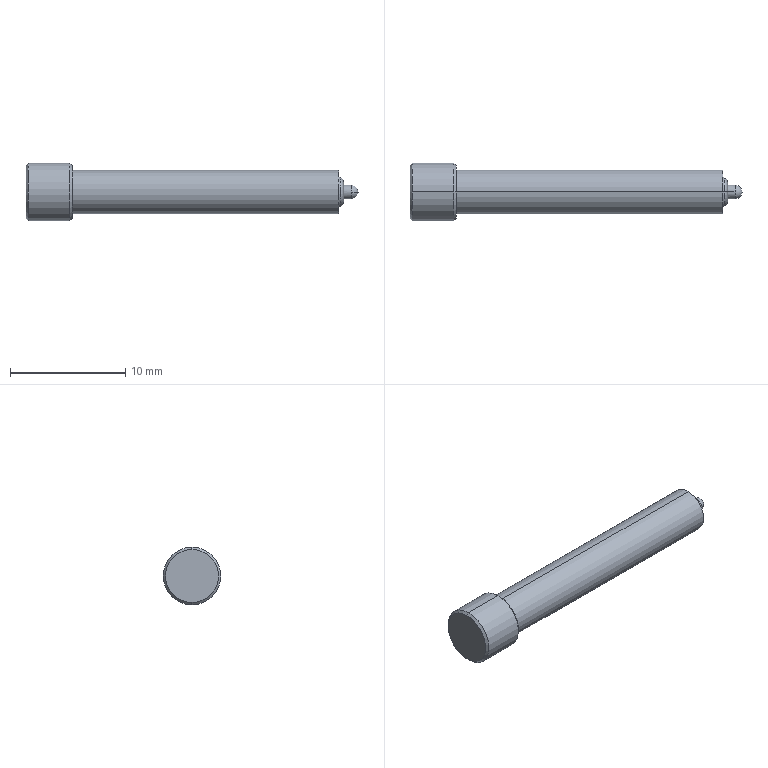Part | STEP file | Riveting punch | 1 solid | 20 faces | box 28.754 x 5 x 5 mm | volume 342.473 mm3 | cylinder 6 | torus 4 | cone 4 | plane 4 | sphere 2 | commonest cylinder face diameters 1.2 x2 3.8 x2 5 x2
STEP:
#1=CARTESIAN_POINT('',(0.,0.,0.));
#2=DIRECTION('',(0.,0.,1.));
#3=DIRECTION('',(1.,0.,0.));
#4=AXIS2_PLACEMENT_3D('',#1,#2,#3);
#5=CARTESIAN_POINT('',(17378.872,34.388,-1.214));
#6=VERTEX_POINT('',#5);
#7=CARTESIAN_POINT('',(17378.72,34.388,-1.85));
#8=VERTEX_POINT('',#7);
#9=CARTESIAN_POINT('',(17379.02,34.388,-1.585));
#10=DIRECTION('',(0.,-1.,0.));
#11=DIRECTION('',(0.,0.,-1.));
#12=AXIS2_PLACEMENT_3D('',#9,#10,#11);
#13=CIRCLE('',#12,0.4);
#14=CARTESIAN_POINT('',(17379.02,34.388,0.));
#15=DIRECTION('',(1.,0.,0.));
#16=DIRECTION('',(0.,0.,-1.));
#17=AXIS2_PLACEMENT_3D('',#14,#15,#16);
#18=TOROIDAL_SURFACE('',#17,1.585,0.4);
#19=CARTESIAN_POINT('',(6.283,0.));
#20=DIRECTION('',(0.,1.));
#21=VECTOR('',#20,1.);
#22=LINE('',#19,#21);
#23=(GEOMETRIC_REPRESENTATION_CONTEXT(2)PARAMETRIC_REPRESENTATION_CONTEXT()REPRESENTATION_CONTEXT('',''));
#24=DEFINITIONAL_REPRESENTATION('',(#22),#23);
#25=PCURVE('',#18,#24);
#26=CARTESIAN_POINT('',(17379.02,34.388,0.));
#27=DIRECTION('',(1.,0.,0.));
#28=DIRECTION('',(0.,0.,-1.));
#29=AXIS2_PLACEMENT_3D('',#26,#27,#28);
#30=TOROIDAL_SURFACE('',#29,1.585,0.4);
#31=CARTESIAN_POINT('',(0.,0.));
#32=DIRECTION('',(0.,1.));
#33=VECTOR('',#32,1.);
#34=LINE('',#31,#33);
#35=(GEOMETRIC_REPRESENTATION_CONTEXT(2)PARAMETRIC_REPRESENTATION_CONTEXT()REPRESENTATION_CONTEXT('',''));
#36=DEFINITIONAL_REPRESENTATION('',(#34),#35);
#37=PCURVE('',#30,#36);
#38=SURFACE_CURVE('',#13,(#25,#37),.PCURVE_S1.);
#39=EDGE_CURVE('',#6,#8,#38,.T.);
#40=ORIENTED_EDGE('',*,*,#39,.T.);
#41=CARTESIAN_POINT('',(17378.72,34.388,1.85));
#42=VERTEX_POINT('',#41);
#43=CARTESIAN_POINT('',(17378.72,34.388,0.));
#44=DIRECTION('',(1.,0.,0.));
#45=DIRECTION('',(0.,0.,-1.));
#46=AXIS2_PLACEMENT_3D('',#43,#44,#45);
#47=CIRCLE('',#46,1.85);
#48=CARTESIAN_POINT('',(0.,5.435));
#49=DIRECTION('',(1.,0.));
#50=VECTOR('',#49,1.);
#51=LINE('',#48,#50);
#52=(GEOMETRIC_REPRESENTATION_CONTEXT(2)PARAMETRIC_REPRESENTATION_CONTEXT()REPRESENTATION_CONTEXT('',''));
#53=DEFINITIONAL_REPRESENTATION('',(#51),#52);
#54=PCURVE('',#18,#53);
#55=CARTESIAN_POINT('',(17378.72,36.238,0.));
#56=DIRECTION('',(1.,0.,0.));
#57=DIRECTION('',(0.,0.,-1.));
#58=AXIS2_PLACEMENT_3D('',#55,#56,#57);
#59=PLANE('',#58);
#60=CARTESIAN_POINT('',(0.,-1.85));
#61=DIRECTION('',(1.,0.));
#62=AXIS2_PLACEMENT_2D('',#60,#61);
#63=CIRCLE('',#62,1.85);
#64=(GEOMETRIC_REPRESENTATION_CONTEXT(2)PARAMETRIC_REPRESENTATION_CONTEXT()REPRESENTATION_CONTEXT('',''));
#65=DEFINITIONAL_REPRESENTATION('',(#63),#64);
#66=PCURVE('',#59,#65);
#67=SURFACE_CURVE('',#47,(#54,#66),.PCURVE_S1.);
#68=EDGE_CURVE('',#42,#8,#67,.T.);
#69=ORIENTED_EDGE('',*,*,#68,.F.);
#70=CARTESIAN_POINT('',(17378.872,34.388,1.214));
#71=VERTEX_POINT('',#70);
#72=CARTESIAN_POINT('',(17379.02,34.388,1.585));
#73=DIRECTION('',(0.,1.,0.));
#74=DIRECTION('',(0.,0.,1.));
#75=AXIS2_PLACEMENT_3D('',#72,#73,#74);
#76=CIRCLE('',#75,0.4);
#77=CARTESIAN_POINT('',(3.142,0.));
#78=DIRECTION('',(0.,1.));
#79=VECTOR('',#78,1.);
#80=LINE('',#77,#79);
#81=(GEOMETRIC_REPRESENTATION_CONTEXT(2)PARAMETRIC_REPRESENTATION_CONTEXT()REPRESENTATION_CONTEXT('',''));
#82=DEFINITIONAL_REPRESENTATION('',(#80),#81);
#83=PCURVE('',#18,#82);
#84=CARTESIAN_POINT('',(3.142,0.));
#85=DIRECTION('',(0.,1.));
#86=VECTOR('',#85,1.);
#87=LINE('',#84,#86);
#88=(GEOMETRIC_REPRESENTATION_CONTEXT(2)PARAMETRIC_REPRESENTATION_CONTEXT()REPRESENTATION_CONTEXT('',''));
#89=DEFINITIONAL_REPRESENTATION('',(#87),#88);
#90=PCURVE('',#30,#89);
#91=SURFACE_CURVE('',#76,(#83,#90),.PCURVE_S1.);
#92=EDGE_CURVE('',#71,#42,#91,.T.);
#93=ORIENTED_EDGE('',*,*,#92,.F.);
#94=CARTESIAN_POINT('',(17378.872,34.388,0.));
#95=DIRECTION('',(1.,0.,0.));
#96=DIRECTION('',(0.,0.,-1.));
#97=AXIS2_PLACEMENT_3D('',#94,#95,#96);
#98=CIRCLE('',#97,1.214);
#99=CARTESIAN_POINT('',(0.,3.521));
#100=DIRECTION('',(1.,0.));
#101=VECTOR('',#100,1.);
#102=LINE('',#99,#101);
#103=(GEOMETRIC_REPRESENTATION_CONTEXT(2)PARAMETRIC_REPRESENTATION_CONTEXT()REPRESENTATION_CONTEXT('',''));
#104=DEFINITIONAL_REPRESENTATION('',(#102),#103);
#105=PCURVE('',#18,#104);
#106=CARTESIAN_POINT('',(17378.723,34.388,0.));
#107=DIRECTION('',(1.,0.,0.));
#108=DIRECTION('',(0.,0.,-1.));
#109=AXIS2_PLACEMENT_3D('',#106,#107,#108);
#110=TOROIDAL_SURFACE('',#109,0.8424,0.4);
#111=CARTESIAN_POINT('',(0.,0.3796));
#112=DIRECTION('',(1.,0.));
#113=VECTOR('',#112,1.);
#114=LINE('',#111,#113);
#115=(GEOMETRIC_REPRESENTATION_CONTEXT(2)PARAMETRIC_REPRESENTATION_CONTEXT()REPRESENTATION_CONTEXT('',''));
#116=DEFINITIONAL_REPRESENTATION('',(#114),#115);
#117=PCURVE('',#110,#116);
#118=SURFACE_CURVE('',#98,(#105,#117),.PCURVE_S1.);
#119=EDGE_CURVE('',#71,#6,#118,.T.);
#120=ORIENTED_EDGE('',*,*,#119,.T.);
#121=EDGE_LOOP('',(#40,#69,#93,#120));
#122=FACE_BOUND('',#121,.F.);
#123=ADVANCED_FACE('',(#122),#18,.F.);
#124=CARTESIAN_POINT('',(17378.872,34.388,0.));
#125=DIRECTION('',(1.,0.,0.));
#126=DIRECTION('',(0.,0.,-1.));
#127=AXIS2_PLACEMENT_3D('',#124,#125,#126);
#128=CIRCLE('',#127,1.214);
#129=CARTESIAN_POINT('',(17378.723,34.388,0.));
#130=DIRECTION('',(1.,0.,0.));
#131=DIRECTION('',(0.,0.,-1.));
#132=AXIS2_PLACEMENT_3D('',#129,#130,#131);
#133=TOROIDAL_SURFACE('',#132,0.8424,0.4);
#134=CARTESIAN_POINT('',(0.,0.3796));
#135=DIRECTION('',(1.,0.));
#136=VECTOR('',#135,1.);
#137=LINE('',#134,#136);
#138=(GEOMETRIC_REPRESENTATION_CONTEXT(2)PARAMETRIC_REPRESENTATION_CONTEXT()REPRESENTATION_CONTEXT('',''));
#139=DEFINITIONAL_REPRESENTATION('',(#137),#138);
#140=PCURVE('',#133,#139);
#141=CARTESIAN_POINT('',(0.,3.521));
#142=DIRECTION('',(1.,0.));
#143=VECTOR('',#142,1.);
#144=LINE('',#141,#143);
#145=(GEOMETRIC_REPRESENTATION_CONTEXT(2)PARAMETRIC_REPRESENTATION_CONTEXT()REPRESENTATION_CONTEXT('',''));
#146=DEFINITIONAL_REPRESENTATION('',(#144),#145);
#147=PCURVE('',#30,#146);
#148=SURFACE_CURVE('',#128,(#140,#147),.PCURVE_S1.);
#149=EDGE_CURVE('',#6,#71,#148,.T.);
#150=ORIENTED_EDGE('',*,*,#149,.T.);
#151=CARTESIAN_POINT('',(17379.123,34.388,0.8424));
#152=VERTEX_POINT('',#151);
#153=CARTESIAN_POINT('',(17378.723,34.388,0.8424));
#154=DIRECTION('',(0.,1.,0.));
#155=DIRECTION('',(0.,0.,1.));
#156=AXIS2_PLACEMENT_3D('',#153,#154,#155);
#157=CIRCLE('',#156,0.4);
#158=CARTESIAN_POINT('',(3.142,0.));
#159=DIRECTION('',(0.,1.));
#160=VECTOR('',#159,1.);
#161=LINE('',#158,#160);
#162=(GEOMETRIC_REPRESENTATION_CONTEXT(2)PARAMETRIC_REPRESENTATION_CONTEXT()REPRESENTATION_CONTEXT('',''));
#163=DEFINITIONAL_REPRESENTATION('',(#161),#162);
#164=PCURVE('',#133,#163);
#165=CARTESIAN_POINT('',(3.142,0.));
#166=DIRECTION('',(0.,1.));
#167=VECTOR('',#166,1.);
#168=LINE('',#165,#167);
#169=(GEOMETRIC_REPRESENTATION_CONTEXT(2)PARAMETRIC_REPRESENTATION_CONTEXT()REPRESENTATION_CONTEXT('',''));
#170=DEFINITIONAL_REPRESENTATION('',(#168),#169);
#171=PCURVE('',#110,#170);
#172=SURFACE_CURVE('',#157,(#164,#171),.PCURVE_S1.);
#173=EDGE_CURVE('',#71,#152,#172,.T.);
#174=ORIENTED_EDGE('',*,*,#173,.T.);
#175=CARTESIAN_POINT('',(17379.123,34.388,-0.8424));
#176=VERTEX_POINT('',#175);
#177=CARTESIAN_POINT('',(17379.123,34.388,0.));
#178=DIRECTION('',(1.,0.,0.));
#179=DIRECTION('',(0.,0.,-1.));
#180=AXIS2_PLACEMENT_3D('',#177,#178,#179);
#181=CIRCLE('',#180,0.8424);
#182=CARTESIAN_POINT('',(0.,1.571));
#183=DIRECTION('',(1.,0.));
#184=VECTOR('',#183,1.);
#185=LINE('',#182,#184);
#186=(GEOMETRIC_REPRESENTATION_CONTEXT(2)PARAMETRIC_REPRESENTATION_CONTEXT()REPRESENTATION_CONTEXT('',''));
#187=DEFINITIONAL_REPRESENTATION('',(#185),#186);
#188=PCURVE('',#133,#187);
#189=CARTESIAN_POINT('',(17379.123,35.231,0.));
#190=DIRECTION('',(1.,0.,0.));
#191=DIRECTION('',(0.,0.,-1.));
#192=AXIS2_PLACEMENT_3D('',#189,#190,#191);
#193=PLANE('',#192);
#194=CARTESIAN_POINT('',(0.,-0.8424));
#195=DIRECTION('',(1.,0.));
#196=AXIS2_PLACEMENT_2D('',#194,#195);
#197=CIRCLE('',#196,0.8424);
#198=(GEOMETRIC_REPRESENTATION_CONTEXT(2)PARAMETRIC_REPRESENTATION_CONTEXT()REPRESENTATION_CONTEXT('',''));
#199=DEFINITIONAL_REPRESENTATION('',(#197),#198);
#200=PCURVE('',#193,#199);
#201=SURFACE_CURVE('',#181,(#188,#200),.PCURVE_S1.);
#202=EDGE_CURVE('',#176,#152,#201,.T.);
#203=ORIENTED_EDGE('',*,*,#202,.F.);
#204=CARTESIAN_POINT('',(17378.723,34.388,-0.8424));
#205=DIRECTION('',(0.,-1.,0.));
#206=DIRECTION('',(0.,0.,-1.));
#207=AXIS2_PLACEMENT_3D('',#204,#205,#206);
#208=CIRCLE('',#207,0.4);
#209=CARTESIAN_POINT('',(0.,0.));
#210=DIRECTION('',(0.,1.));
#211=VECTOR('',#210,1.);
#212=LINE('',#209,#211);
#213=(GEOMETRIC_REPRESENTATION_CONTEXT(2)PARAMETRIC_REPRESENTATION_CONTEXT()REPRESENTATION_CONTEXT('',''));
#214=DEFINITIONAL_REPRESENTATION('',(#212),#213);
#215=PCURVE('',#133,#214);
#216=CARTESIAN_POINT('',(6.283,0.));
#217=DIRECTION('',(0.,1.));
#218=VECTOR('',#217,1.);
#219=LINE('',#216,#218);
#220=(GEOMETRIC_REPRESENTATION_CONTEXT(2)PARAMETRIC_REPRESENTATION_CONTEXT()REPRESENTATION_CONTEXT('',''));
#221=DEFINITIONAL_REPRESENTATION('',(#219),#220);
#222=PCURVE('',#110,#221);
#223=SURFACE_CURVE('',#208,(#215,#222),.PCURVE_S1.);
#224=EDGE_CURVE('',#6,#176,#223,.T.);
#225=ORIENTED_EDGE('',*,*,#224,.F.);
#226=EDGE_LOOP('',(#150,#174,#203,#225));
#227=FACE_BOUND('',#226,.T.);
#228=ADVANCED_FACE('',(#227),#133,.T.);
#229=CARTESIAN_POINT('',(17379.123,34.388,-0.6));
#230=VERTEX_POINT('',#229);
#231=CARTESIAN_POINT('',(17379.123,34.388,0.6));
#232=VERTEX_POINT('',#231);
#233=CARTESIAN_POINT('',(17379.123,34.388,0.));
#234=DIRECTION('',(1.,0.,0.));
#235=DIRECTION('',(0.,0.,-1.));
#236=AXIS2_PLACEMENT_3D('',#233,#234,#235);
#237=CIRCLE('',#236,0.6);
#238=CARTESIAN_POINT('',(17380.373,34.388,0.));
#239=DIRECTION('',(1.,0.,0.));
#240=DIRECTION('',(0.,0.,-1.));
#241=AXIS2_PLACEMENT_3D('',#238,#239,#240);
#242=CYLINDRICAL_SURFACE('',#241,0.6);
#243=CARTESIAN_POINT('',(0.,-1.25));
#244=DIRECTION('',(1.,0.));
#245=VECTOR('',#244,1.);
#246=LINE('',#243,#245);
#247=(GEOMETRIC_REPRESENTATION_CONTEXT(2)PARAMETRIC_REPRESENTATION_CONTEXT()REPRESENTATION_CONTEXT('',''));
#248=DEFINITIONAL_REPRESENTATION('',(#246),#247);
#249=PCURVE('',#242,#248);
#250=CARTESIAN_POINT('',(0.,-0.8424));
#251=DIRECTION('',(1.,0.));
#252=AXIS2_PLACEMENT_2D('',#250,#251);
#253=CIRCLE('',#252,0.6);
#254=(GEOMETRIC_REPRESENTATION_CONTEXT(2)PARAMETRIC_REPRESENTATION_CONTEXT()REPRESENTATION_CONTEXT('',''));
#255=DEFINITIONAL_REPRESENTATION('',(#253),#254);
#256=PCURVE('',#193,#255);
#257=SURFACE_CURVE('',#237,(#249,#256),.PCURVE_S1.);
#258=EDGE_CURVE('',#230,#232,#257,.T.);
#259=ORIENTED_EDGE('',*,*,#258,.T.);
#260=CARTESIAN_POINT('',(17379.773,34.388,0.6));
#261=VERTEX_POINT('',#260);
#262=CARTESIAN_POINT('',(17380.373,34.388,0.6));
#263=DIRECTION('',(1.,0.,0.));
#264=VECTOR('',#263,1.);
#265=LINE('',#262,#264);
#266=CARTESIAN_POINT('',(3.142,0.));
#267=DIRECTION('',(0.,1.));
#268=VECTOR('',#267,1.);
#269=LINE('',#266,#268);
#270=(GEOMETRIC_REPRESENTATION_CONTEXT(2)PARAMETRIC_REPRESENTATION_CONTEXT()REPRESENTATION_CONTEXT('',''));
#271=DEFINITIONAL_REPRESENTATION('',(#269),#270);
#272=PCURVE('',#242,#271);
#273=CARTESIAN_POINT('',(17380.373,34.388,0.));
#274=DIRECTION('',(1.,0.,0.));
#275=DIRECTION('',(0.,0.,-1.));
#276=AXIS2_PLACEMENT_3D('',#273,#274,#275);
#277=CYLINDRICAL_SURFACE('',#276,0.6);
#278=CARTESIAN_POINT('',(3.142,0.));
#279=DIRECTION('',(0.,1.));
#280=VECTOR('',#279,1.);
#281=LINE('',#278,#280);
#282=(GEOMETRIC_REPRESENTATION_CONTEXT(2)PARAMETRIC_REPRESENTATION_CONTEXT()REPRESENTATION_CONTEXT('',''));
#283=DEFINITIONAL_REPRESENTATION('',(#281),#282);
#284=PCURVE('',#277,#283);
#285=SURFACE_CURVE('',#265,(#272,#284),.PCURVE_S1.);
#286=EDGE_CURVE('',#232,#261,#285,.T.);
#287=ORIENTED_EDGE('',*,*,#286,.T.);
#288=CARTESIAN_POINT('',(17379.773,34.988,0.));
#289=VERTEX_POINT('',#288);
#290=CARTESIAN_POINT('',(17379.773,34.388,0.));
#291=DIRECTION('',(1.,0.,0.));
#292=DIRECTION('',(0.,0.,-1.));
#293=AXIS2_PLACEMENT_3D('',#290,#291,#292);
#294=CIRCLE('',#293,0.6);
#295=CARTESIAN_POINT('',(0.,-0.6));
#296=DIRECTION('',(1.,0.));
#297=VECTOR('',#296,1.);
#298=LINE('',#295,#297);
#299=(GEOMETRIC_REPRESENTATION_CONTEXT(2)PARAMETRIC_REPRESENTATION_CONTEXT()REPRESENTATION_CONTEXT('',''));
#300=DEFINITIONAL_REPRESENTATION('',(#298),#299);
#301=PCURVE('',#242,#300);
#302=CARTESIAN_POINT('',(17379.773,34.388,0.));
#303=DIRECTION('',(0.,0.,1.));
#304=DIRECTION('',(0.,1.,0.));
#305=AXIS2_PLACEMENT_3D('',#302,#303,#304);
#306=SPHERICAL_SURFACE('',#305,0.6);
#307=CARTESIAN_POINT('',(6.283,-1.571));
#308=DIRECTION('',(0.,1.));
#309=VECTOR('',#308,1.);
#310=LINE('',#307,#309);
#311=(GEOMETRIC_REPRESENTATION_CONTEXT(2)PARAMETRIC_REPRESENTATION_CONTEXT()REPRESENTATION_CONTEXT('',''));
#312=DEFINITIONAL_REPRESENTATION('',(#310),#311);
#313=PCURVE('',#306,#312);
#314=SURFACE_CURVE('',#294,(#301,#313),.PCURVE_S1.);
#315=EDGE_CURVE('',#289,#261,#314,.T.);
#316=ORIENTED_EDGE('',*,*,#315,.F.);
#317=CARTESIAN_POINT('',(17379.773,34.388,-0.6));
#318=VERTEX_POINT('',#317);
#319=CARTESIAN_POINT('',(17379.773,34.388,0.));
#320=DIRECTION('',(1.,0.,0.));
#321=DIRECTION('',(0.,0.,-1.));
#322=AXIS2_PLACEMENT_3D('',#319,#320,#321);
#323=CIRCLE('',#322,0.6);
#324=CARTESIAN_POINT('',(0.,-0.6));
#325=DIRECTION('',(1.,0.));
#326=VECTOR('',#325,1.);
#327=LINE('',#324,#326);
#328=(GEOMETRIC_REPRESENTATION_CONTEXT(2)PARAMETRIC_REPRESENTATION_CONTEXT()REPRESENTATION_CONTEXT('',''));
#329=DEFINITIONAL_REPRESENTATION('',(#327),#328);
#330=PCURVE('',#242,#329);
#331=CARTESIAN_POINT('',(17379.773,34.388,0.));
#332=DIRECTION('',(0.,0.,1.));
#333=DIRECTION('',(0.,1.,0.));
#334=AXIS2_PLACEMENT_3D('',#331,#332,#333);
#335=SPHERICAL_SURFACE('',#334,0.6);
#336=CARTESIAN_POINT('',(6.283,-1.571));
#337=DIRECTION('',(0.,1.));
#338=VECTOR('',#337,1.);
#339=LINE('',#336,#338);
#340=(GEOMETRIC_REPRESENTATION_CONTEXT(2)PARAMETRIC_REPRESENTATION_CONTEXT()REPRESENTATION_CONTEXT('',''));
#341=DEFINITIONAL_REPRESENTATION('',(#339),#340);
#342=PCURVE('',#335,#341);
#343=SURFACE_CURVE('',#323,(#330,#342),.PCURVE_S1.);
#344=EDGE_CURVE('',#318,#289,#343,.T.);
#345=ORIENTED_EDGE('',*,*,#344,.F.);
#346=CARTESIAN_POINT('',(17380.373,34.388,-0.6));
#347=DIRECTION('',(1.,0.,0.));
#348=VECTOR('',#347,1.);
#349=LINE('',#346,#348);
#350=CARTESIAN_POINT('',(0.,0.));
#351=DIRECTION('',(0.,1.));
#352=VECTOR('',#351,1.);
#353=LINE('',#350,#352);
#354=(GEOMETRIC_REPRESENTATION_CONTEXT(2)PARAMETRIC_REPRESENTATION_CONTEXT()REPRESENTATION_CONTEXT('',''));
#355=DEFINITIONAL_REPRESENTATION('',(#353),#354);
#356=PCURVE('',#242,#355);
#357=CARTESIAN_POINT('',(6.283,0.));
#358=DIRECTION('',(0.,1.));
#359=VECTOR('',#358,1.);
#360=LINE('',#357,#359);
#361=(GEOMETRIC_REPRESENTATION_CONTEXT(2)PARAMETRIC_REPRESENTATION_CONTEXT()REPRESENTATION_CONTEXT('',''));
#362=DEFINITIONAL_REPRESENTATION('',(#360),#361);
#363=PCURVE('',#277,#362);
#364=SURFACE_CURVE('',#349,(#356,#363),.PCURVE_S1.);
#365=EDGE_CURVE('',#230,#318,#364,.T.);
#366=ORIENTED_EDGE('',*,*,#365,.F.);
#367=EDGE_LOOP('',(#259,#287,#316,#345,#366));
#368=FACE_BOUND('',#367,.T.);
#369=ADVANCED_FACE('',(#368),#242,.T.);
#370=ORIENTED_EDGE('',*,*,#315,.T.);
#371=CARTESIAN_POINT('',(17379.773,33.788,0.));
#372=VERTEX_POINT('',#371);
#373=CARTESIAN_POINT('',(17379.773,34.388,0.));
#374=DIRECTION('',(1.,0.,0.));
#375=DIRECTION('',(0.,0.,-1.));
#376=AXIS2_PLACEMENT_3D('',#373,#374,#375);
#377=CIRCLE('',#376,0.6);
#378=CARTESIAN_POINT('',(3.142,1.571));
#379=CARTESIAN_POINT('',(3.142,1.547));
#380=CARTESIAN_POINT('',(3.142,1.499));
#381=CARTESIAN_POINT('',(3.142,1.428));
#382=CARTESIAN_POINT('',(3.142,1.357));
#383=CARTESIAN_POINT('',(3.142,1.285));
#384=CARTESIAN_POINT('',(3.142,1.214));
#385=CARTESIAN_POINT('',(3.142,1.142));
#386=CARTESIAN_POINT('',(3.142,1.071));
#387=CARTESIAN_POINT('',(3.142,0.9996));
#388=CARTESIAN_POINT('',(3.142,0.9282));
#389=CARTESIAN_POINT('',(3.142,0.8568));
#390=CARTESIAN_POINT('',(3.142,0.7854));
#391=CARTESIAN_POINT('',(3.142,0.714));
#392=CARTESIAN_POINT('',(3.142,0.6426));
#393=CARTESIAN_POINT('',(3.142,0.5712));
#394=CARTESIAN_POINT('',(3.142,0.4998));
#395=CARTESIAN_POINT('',(3.142,0.4284));
#396=CARTESIAN_POINT('',(3.142,0.357));
#397=CARTESIAN_POINT('',(3.142,0.2856));
#398=CARTESIAN_POINT('',(3.142,0.2142));
#399=CARTESIAN_POINT('',(3.142,0.1428));
#400=CARTESIAN_POINT('',(3.142,0.0714));
#401=CARTESIAN_POINT('',(3.142,0.0238));
#402=CARTESIAN_POINT('',(3.142,0.));
#403=B_SPLINE_CURVE_WITH_KNOTS('',3,(#378,#379,#380,#381,#382,#383,#384,#385,#386,#387,#388,#389,#390,#391,#392,#393,#394,#395,#396,#397,#398,#399,#400,#401,#402),.UNSPECIFIED.,.F.,.F.,(4,1,1,1,1,1,1,1,1,1,1,1,1,1,1,1,1,1,1,1,1,1,4),(3.142,3.213,3.284,3.356,3.427,3.499,3.57,3.641,3.713,3.784,3.856,3.927,3.998,4.07,4.141,4.213,4.284,4.355,4.427,4.498,4.57,4.641,4.712),.QUASI_UNIFORM_KNOTS.);
#404=(GEOMETRIC_REPRESENTATION_CONTEXT(2)PARAMETRIC_REPRESENTATION_CONTEXT()REPRESENTATION_CONTEXT('',''));
#405=DEFINITIONAL_REPRESENTATION('',(#403),#404);
#406=PCURVE('',#306,#405);
#407=CARTESIAN_POINT('',(0.,-0.6));
#408=DIRECTION('',(1.,0.));
#409=VECTOR('',#408,1.);
#410=LINE('',#407,#409);
#411=(GEOMETRIC_REPRESENTATION_CONTEXT(2)PARAMETRIC_REPRESENTATION_CONTEXT()REPRESENTATION_CONTEXT('',''));
#412=DEFINITIONAL_REPRESENTATION('',(#410),#411);
#413=PCURVE('',#277,#412);
#414=SURFACE_CURVE('',#377,(#406,#413),.PCURVE_S1.);
#415=EDGE_CURVE('',#261,#372,#414,.T.);
#416=ORIENTED_EDGE('',*,*,#415,.T.);
#417=CARTESIAN_POINT('',(17380.373,34.388,0.));
#418=VERTEX_POINT('',#417);
#419=CARTESIAN_POINT('',(17379.773,34.388,0.));
#420=DIRECTION('',(0.,0.,1.));
#421=DIRECTION('',(0.,-1.,0.));
#422=AXIS2_PLACEMENT_3D('',#419,#420,#421);
#423=CIRCLE('',#422,0.6);
#424=CARTESIAN_POINT('',(3.142,0.));
#425=DIRECTION('',(1.,0.));
#426=VECTOR('',#425,1.);
#427=LINE('',#424,#426);
#428=(GEOMETRIC_REPRESENTATION_CONTEXT(2)PARAMETRIC_REPRESENTATION_CONTEXT()REPRESENTATION_CONTEXT('',''));
#429=DEFINITIONAL_REPRESENTATION('',(#427),#428);
#430=PCURVE('',#306,#429);
#431=CARTESIAN_POINT('',(3.142,0.));
#432=DIRECTION('',(1.,0.));
#433=VECTOR('',#432,1.);
#434=LINE('',#431,#433);
#435=(GEOMETRIC_REPRESENTATION_CONTEXT(2)PARAMETRIC_REPRESENTATION_CONTEXT()REPRESENTATION_CONTEXT('',''));
#436=DEFINITIONAL_REPRESENTATION('',(#434),#435);
#437=PCURVE('',#335,#436);
#438=SURFACE_CURVE('',#423,(#430,#437),.PCURVE_S1.);
#439=EDGE_CURVE('',#372,#418,#438,.T.);
#440=ORIENTED_EDGE('',*,*,#439,.T.);
#441=CARTESIAN_POINT('',(17379.773,34.388,0.));
#442=DIRECTION('',(0.,0.,-1.));
#443=DIRECTION('',(-1.,0.,0.));
#444=AXIS2_PLACEMENT_3D('',#441,#442,#443);
#445=CIRCLE('',#444,0.6);
#446=CARTESIAN_POINT('',(6.283,0.));
#447=CARTESIAN_POINT('',(6.259,0.));
#448=CARTESIAN_POINT('',(6.212,0.));
#449=CARTESIAN_POINT('',(6.14,0.));
#450=CARTESIAN_POINT('',(6.069,0.));
#451=CARTESIAN_POINT('',(5.998,0.));
#452=CARTESIAN_POINT('',(5.926,0.));
#453=CARTESIAN_POINT('',(5.855,0.));
#454=CARTESIAN_POINT('',(5.783,0.));
#455=CARTESIAN_POINT('',(5.712,0.));
#456=CARTESIAN_POINT('',(5.641,0.));
#457=CARTESIAN_POINT('',(5.569,0.));
#458=CARTESIAN_POINT('',(5.498,0.));
#459=CARTESIAN_POINT('',(5.426,0.));
#460=CARTESIAN_POINT('',(5.355,0.));
#461=CARTESIAN_POINT('',(5.284,0.));
#462=CARTESIAN_POINT('',(5.212,0.));
#463=CARTESIAN_POINT('',(5.141,0.));
#464=CARTESIAN_POINT('',(5.069,0.));
#465=CARTESIAN_POINT('',(4.998,0.));
#466=CARTESIAN_POINT('',(4.927,0.));
#467=CARTESIAN_POINT('',(4.855,0.));
#468=CARTESIAN_POINT('',(4.784,0.));
#469=CARTESIAN_POINT('',(4.736,0.));
#470=CARTESIAN_POINT('',(4.712,0.));
#471=B_SPLINE_CURVE_WITH_KNOTS('',3,(#446,#447,#448,#449,#450,#451,#452,#453,#454,#455,#456,#457,#458,#459,#460,#461,#462,#463,#464,#465,#466,#467,#468,#469,#470),.UNSPECIFIED.,.F.,.F.,(4,1,1,1,1,1,1,1,1,1,1,1,1,1,1,1,1,1,1,1,1,1,4),(1.571,1.642,1.714,1.785,1.856,1.928,1.999,2.071,2.142,2.213,2.285,2.356,2.428,2.499,2.57,2.642,2.713,2.785,2.856,2.927,2.999,3.07,3.142),.QUASI_UNIFORM_KNOTS.);
#472=(GEOMETRIC_REPRESENTATION_CONTEXT(2)PARAMETRIC_REPRESENTATION_CONTEXT()REPRESENTATION_CONTEXT('',''));
#473=DEFINITIONAL_REPRESENTATION('',(#471),#472);
#474=PCURVE('',#306,#473);
#475=CARTESIAN_POINT('',(6.283,0.));
#476=CARTESIAN_POINT('',(6.259,0.));
#477=CARTESIAN_POINT('',(6.212,0.));
#478=CARTESIAN_POINT('',(6.14,0.));
#479=CARTESIAN_POINT('',(6.069,0.));
#480=CARTESIAN_POINT('',(5.998,0.));
#481=CARTESIAN_POINT('',(5.926,0.));
#482=CARTESIAN_POINT('',(5.855,0.));
#483=CARTESIAN_POINT('',(5.783,0.));
#484=CARTESIAN_POINT('',(5.712,0.));
#485=CARTESIAN_POINT('',(5.641,0.));
#486=CARTESIAN_POINT('',(5.569,0.));
#487=CARTESIAN_POINT('',(5.498,0.));
#488=CARTESIAN_POINT('',(5.426,0.));
#489=CARTESIAN_POINT('',(5.355,0.));
#490=CARTESIAN_POINT('',(5.284,0.));
#491=CARTESIAN_POINT('',(5.212,0.));
#492=CARTESIAN_POINT('',(5.141,0.));
#493=CARTESIAN_POINT('',(5.069,0.));
#494=CARTESIAN_POINT('',(4.998,0.));
#495=CARTESIAN_POINT('',(4.927,0.));
#496=CARTESIAN_POINT('',(4.855,0.));
#497=CARTESIAN_POINT('',(4.784,0.));
#498=CARTESIAN_POINT('',(4.736,0.));
#499=CARTESIAN_POINT('',(4.712,0.));
#500=B_SPLINE_CURVE_WITH_KNOTS('',3,(#475,#476,#477,#478,#479,#480,#481,#482,#483,#484,#485,#486,#487,#488,#489,#490,#491,#492,#493,#494,#495,#496,#497,#498,#499),.UNSPECIFIED.,.F.,.F.,(4,1,1,1,1,1,1,1,1,1,1,1,1,1,1,1,1,1,1,1,1,1,4),(1.571,1.642,1.714,1.785,1.856,1.928,1.999,2.071,2.142,2.213,2.285,2.356,2.428,2.499,2.57,2.642,2.713,2.785,2.856,2.927,2.999,3.07,3.142),.QUASI_UNIFORM_KNOTS.);
#501=(GEOMETRIC_REPRESENTATION_CONTEXT(2)PARAMETRIC_REPRESENTATION_CONTEXT()REPRESENTATION_CONTEXT('',''));
#502=DEFINITIONAL_REPRESENTATION('',(#500),#501);
#503=PCURVE('',#335,#502);
#504=SURFACE_CURVE('',#445,(#474,#503),.PCURVE_S1.);
#505=EDGE_CURVE('',#289,#418,#504,.T.);
#506=ORIENTED_EDGE('',*,*,#505,.F.);
#507=EDGE_LOOP('',(#370,#416,#440,#506));
#508=FACE_BOUND('',#507,.T.);
#509=ADVANCED_FACE('',(#508),#306,.T.);
#510=CARTESIAN_POINT('',(17351.62,34.388,-2.3));
#511=VERTEX_POINT('',#510);
#512=CARTESIAN_POINT('',(17351.62,34.388,2.3));
#513=VERTEX_POINT('',#512);
#514=CARTESIAN_POINT('',(17351.62,34.388,0.));
#515=DIRECTION('',(1.,0.,0.));
#516=DIRECTION('',(0.,0.,-1.));
#517=AXIS2_PLACEMENT_3D('',#514,#515,#516);
#518=CIRCLE('',#517,2.3);
#519=CARTESIAN_POINT('',(17351.82,34.388,0.));
#520=DIRECTION('',(1.,0.,0.));
#521=DIRECTION('',(0.,0.,-1.));
#522=AXIS2_PLACEMENT_3D('',#519,#520,#521);
#523=CONICAL_SURFACE('',#522,2.5,0.7854);
#524=CARTESIAN_POINT('',(0.,-0.2));
#525=DIRECTION('',(1.,0.));
#526=VECTOR('',#525,1.);
#527=LINE('',#524,#526);
#528=(GEOMETRIC_REPRESENTATION_CONTEXT(2)PARAMETRIC_REPRESENTATION_CONTEXT()REPRESENTATION_CONTEXT('',''));
#529=DEFINITIONAL_REPRESENTATION('',(#527),#528);
#530=PCURVE('',#523,#529);
#531=CARTESIAN_POINT('',(17351.62,36.688,0.));
#532=DIRECTION('',(-1.,0.,0.));
#533=DIRECTION('',(0.,0.,1.));
#534=AXIS2_PLACEMENT_3D('',#531,#532,#533);
#535=PLANE('',#534);
#536=CARTESIAN_POINT('',(-2.3,-2.3));
#537=CARTESIAN_POINT('',(-2.3,1.684));
#538=CARTESIAN_POINT('',(1.15,-0.3081));
#539=CARTESIAN_POINT('',(4.6,-2.3));
#540=CARTESIAN_POINT('',(1.15,-4.292));
#541=CARTESIAN_POINT('',(-2.3,-6.284));
#542=CARTESIAN_POINT('',(-2.3,-2.3));
#543=(BOUNDED_CURVE()B_SPLINE_CURVE(2,(#536,#537,#538,#539,#540,#541,#542),.UNSPECIFIED.,.T.,.F.)B_SPLINE_CURVE_WITH_KNOTS((1,2,2,2,2,1),(-2.094,0.,2.094,4.189,6.283,8.378),.UNSPECIFIED.)CURVE()GEOMETRIC_REPRESENTATION_ITEM()RATIONAL_B_SPLINE_CURVE((1.,0.5,1.,0.5,1.,0.5,1.))REPRESENTATION_ITEM(''));
#544=(GEOMETRIC_REPRESENTATION_CONTEXT(2)PARAMETRIC_REPRESENTATION_CONTEXT()REPRESENTATION_CONTEXT('',''));
#545=DEFINITIONAL_REPRESENTATION('',(#543),#544);
#546=PCURVE('',#535,#545);
#547=SURFACE_CURVE('',#518,(#530,#546),.PCURVE_S1.);
#548=EDGE_CURVE('',#511,#513,#547,.T.);
#549=ORIENTED_EDGE('',*,*,#548,.T.);
#550=CARTESIAN_POINT('',(17351.82,34.388,2.5));
#551=VERTEX_POINT('',#550);
#552=CARTESIAN_POINT('',(17351.82,34.388,2.5));
#553=DIRECTION('',(0.7071,0.,0.7071));
#554=VECTOR('',#553,1.);
#555=LINE('',#552,#554);
#556=CARTESIAN_POINT('',(3.142,0.));
#557=DIRECTION('',(0.,1.));
#558=VECTOR('',#557,1.);
#559=LINE('',#556,#558);
#560=(GEOMETRIC_REPRESENTATION_CONTEXT(2)PARAMETRIC_REPRESENTATION_CONTEXT()REPRESENTATION_CONTEXT('',''));
#561=DEFINITIONAL_REPRESENTATION('',(#559),#560);
#562=PCURVE('',#523,#561);
#563=CARTESIAN_POINT('',(17351.82,34.388,0.));
#564=DIRECTION('',(1.,0.,0.));
#565=DIRECTION('',(0.,0.,-1.));
#566=AXIS2_PLACEMENT_3D('',#563,#564,#565);
#567=CONICAL_SURFACE('',#566,2.5,0.7854);
#568=CARTESIAN_POINT('',(3.142,0.));
#569=DIRECTION('',(0.,1.));
#570=VECTOR('',#569,1.);
#571=LINE('',#568,#570);
#572=(GEOMETRIC_REPRESENTATION_CONTEXT(2)PARAMETRIC_REPRESENTATION_CONTEXT()REPRESENTATION_CONTEXT('',''));
#573=DEFINITIONAL_REPRESENTATION('',(#571),#572);
#574=PCURVE('',#567,#573);
#575=SURFACE_CURVE('',#555,(#562,#574),.PCURVE_S1.);
#576=EDGE_CURVE('',#513,#551,#575,.T.);
#577=ORIENTED_EDGE('',*,*,#576,.T.);
#578=CARTESIAN_POINT('',(17351.82,34.388,-2.5));
#579=VERTEX_POINT('',#578);
#580=CARTESIAN_POINT('',(17351.82,34.388,0.));
#581=DIRECTION('',(1.,0.,0.));
#582=DIRECTION('',(0.,0.,-1.));
#583=AXIS2_PLACEMENT_3D('',#580,#581,#582);
#584=CIRCLE('',#583,2.5);
#585=CARTESIAN_POINT('',(0.,0.));
#586=DIRECTION('',(1.,0.));
#587=VECTOR('',#586,1.);
#588=LINE('',#585,#587);
#589=(GEOMETRIC_REPRESENTATION_CONTEXT(2)PARAMETRIC_REPRESENTATION_CONTEXT()REPRESENTATION_CONTEXT('',''));
#590=DEFINITIONAL_REPRESENTATION('',(#588),#589);
#591=PCURVE('',#523,#590);
#592=CARTESIAN_POINT('',(17380.373,34.388,0.));
#593=DIRECTION('',(1.,0.,0.));
#594=DIRECTION('',(0.,0.,-1.));
#595=AXIS2_PLACEMENT_3D('',#592,#593,#594);
#596=CYLINDRICAL_SURFACE('',#595,2.5);
#597=CARTESIAN_POINT('',(0.,-28.554));
#598=DIRECTION('',(1.,0.));
#599=VECTOR('',#598,1.);
#600=LINE('',#597,#599);
#601=(GEOMETRIC_REPRESENTATION_CONTEXT(2)PARAMETRIC_REPRESENTATION_CONTEXT()REPRESENTATION_CONTEXT('',''));
#602=DEFINITIONAL_REPRESENTATION('',(#600),#601);
#603=PCURVE('',#596,#602);
#604=SURFACE_CURVE('',#584,(#591,#603),.PCURVE_S1.);
#605=EDGE_CURVE('',#579,#551,#604,.T.);
#606=ORIENTED_EDGE('',*,*,#605,.F.);
#607=CARTESIAN_POINT('',(17351.82,34.388,-2.5));
#608=DIRECTION('',(0.7071,0.,-0.7071));
#609=VECTOR('',#608,1.);
#610=LINE('',#607,#609);
#611=CARTESIAN_POINT('',(0.,0.));
#612=DIRECTION('',(0.,1.));
#613=VECTOR('',#612,1.);
#614=LINE('',#611,#613);
#615=(GEOMETRIC_REPRESENTATION_CONTEXT(2)PARAMETRIC_REPRESENTATION_CONTEXT()REPRESENTATION_CONTEXT('',''));
#616=DEFINITIONAL_REPRESENTATION('',(#614),#615);
#617=PCURVE('',#523,#616);
#618=CARTESIAN_POINT('',(6.283,0.));
#619=DIRECTION('',(0.,1.));
#620=VECTOR('',#619,1.);
#621=LINE('',#618,#620);
#622=(GEOMETRIC_REPRESENTATION_CONTEXT(2)PARAMETRIC_REPRESENTATION_CONTEXT()REPRESENTATION_CONTEXT('',''));
#623=DEFINITIONAL_REPRESENTATION('',(#621),#622);
#624=PCURVE('',#567,#623);
#625=SURFACE_CURVE('',#610,(#617,#624),.PCURVE_S1.);
#626=EDGE_CURVE('',#511,#579,#625,.T.);
#627=ORIENTED_EDGE('',*,*,#626,.F.);
#628=EDGE_LOOP('',(#549,#577,#606,#627));
#629=FACE_BOUND('',#628,.T.);
#630=ADVANCED_FACE('',(#629),#523,.T.);
#631=ORIENTED_EDGE('',*,*,#605,.T.);
#632=CARTESIAN_POINT('',(17355.42,34.388,2.5));
#633=VERTEX_POINT('',#632);
#634=CARTESIAN_POINT('',(17380.373,34.388,2.5));
#635=DIRECTION('',(1.,0.,0.));
#636=VECTOR('',#635,1.);
#637=LINE('',#634,#636);
#638=CARTESIAN_POINT('',(3.142,0.));
#639=DIRECTION('',(0.,1.));
#640=VECTOR('',#639,1.);
#641=LINE('',#638,#640);
#642=(GEOMETRIC_REPRESENTATION_CONTEXT(2)PARAMETRIC_REPRESENTATION_CONTEXT()REPRESENTATION_CONTEXT('',''));
#643=DEFINITIONAL_REPRESENTATION('',(#641),#642);
#644=PCURVE('',#596,#643);
#645=CARTESIAN_POINT('',(17380.373,34.388,0.));
#646=DIRECTION('',(1.,0.,0.));
#647=DIRECTION('',(0.,0.,-1.));
#648=AXIS2_PLACEMENT_3D('',#645,#646,#647);
#649=CYLINDRICAL_SURFACE('',#648,2.5);
#650=CARTESIAN_POINT('',(3.142,0.));
#651=DIRECTION('',(0.,1.));
#652=VECTOR('',#651,1.);
#653=LINE('',#650,#652);
#654=(GEOMETRIC_REPRESENTATION_CONTEXT(2)PARAMETRIC_REPRESENTATION_CONTEXT()REPRESENTATION_CONTEXT('',''));
#655=DEFINITIONAL_REPRESENTATION('',(#653),#654);
#656=PCURVE('',#649,#655);
#657=SURFACE_CURVE('',#637,(#644,#656),.PCURVE_S1.);
#658=EDGE_CURVE('',#551,#633,#657,.T.);
#659=ORIENTED_EDGE('',*,*,#658,.T.);
#660=CARTESIAN_POINT('',(17355.42,34.388,-2.5));
#661=VERTEX_POINT('',#660);
#662=CARTESIAN_POINT('',(17355.42,34.388,0.));
#663=DIRECTION('',(1.,0.,0.));
#664=DIRECTION('',(0.,0.,-1.));
#665=AXIS2_PLACEMENT_3D('',#662,#663,#664);
#666=CIRCLE('',#665,2.5);
#667=CARTESIAN_POINT('',(0.,-24.954));
#668=DIRECTION('',(1.,0.));
#669=VECTOR('',#668,1.);
#670=LINE('',#667,#669);
#671=(GEOMETRIC_REPRESENTATION_CONTEXT(2)PARAMETRIC_REPRESENTATION_CONTEXT()REPRESENTATION_CONTEXT('',''));
#672=DEFINITIONAL_REPRESENTATION('',(#670),#671);
#673=PCURVE('',#596,#672);
#674=CARTESIAN_POINT('',(17355.62,34.388,0.));
#675=DIRECTION('',(-1.,0.,0.));
#676=DIRECTION('',(0.,0.,1.));
#677=AXIS2_PLACEMENT_3D('',#674,#675,#676);
#678=CONICAL_SURFACE('',#677,2.3,0.7854);
#679=CARTESIAN_POINT('',(3.142,0.2));
#680=DIRECTION('',(-1.,0.));
#681=VECTOR('',#680,1.);
#682=LINE('',#679,#681);
#683=(GEOMETRIC_REPRESENTATION_CONTEXT(2)PARAMETRIC_REPRESENTATION_CONTEXT()REPRESENTATION_CONTEXT('',''));
#684=DEFINITIONAL_REPRESENTATION('',(#682),#683);
#685=PCURVE('',#678,#684);
#686=SURFACE_CURVE('',#666,(#673,#685),.PCURVE_S1.);
#687=EDGE_CURVE('',#661,#633,#686,.T.);
#688=ORIENTED_EDGE('',*,*,#687,.F.);
#689=CARTESIAN_POINT('',(17380.373,34.388,-2.5));
#690=DIRECTION('',(1.,0.,0.));
#691=VECTOR('',#690,1.);
#692=LINE('',#689,#691);
#693=CARTESIAN_POINT('',(0.,0.));
#694=DIRECTION('',(0.,1.));
#695=VECTOR('',#694,1.);
#696=LINE('',#693,#695);
#697=(GEOMETRIC_REPRESENTATION_CONTEXT(2)PARAMETRIC_REPRESENTATION_CONTEXT()REPRESENTATION_CONTEXT('',''));
#698=DEFINITIONAL_REPRESENTATION('',(#696),#697);
#699=PCURVE('',#596,#698);
#700=CARTESIAN_POINT('',(6.283,0.));
#701=DIRECTION('',(0.,1.));
#702=VECTOR('',#701,1.);
#703=LINE('',#700,#702);
#704=(GEOMETRIC_REPRESENTATION_CONTEXT(2)PARAMETRIC_REPRESENTATION_CONTEXT()REPRESENTATION_CONTEXT('',''));
#705=DEFINITIONAL_REPRESENTATION('',(#703),#704);
#706=PCURVE('',#649,#705);
#707=SURFACE_CURVE('',#692,(#699,#706),.PCURVE_S1.);
#708=EDGE_CURVE('',#579,#661,#707,.T.);
#709=ORIENTED_EDGE('',*,*,#708,.F.);
#710=EDGE_LOOP('',(#631,#659,#688,#709));
#711=FACE_BOUND('',#710,.T.);
#712=ADVANCED_FACE('',(#711),#596,.T.);
#713=CARTESIAN_POINT('',(17355.62,34.388,-2.3));
#714=VERTEX_POINT('',#713);
#715=CARTESIAN_POINT('',(17355.62,34.388,2.3));
#716=VERTEX_POINT('',#715);
#717=CARTESIAN_POINT('',(17355.62,34.388,0.));
#718=DIRECTION('',(1.,0.,0.));
#719=DIRECTION('',(0.,0.,-1.));
#720=AXIS2_PLACEMENT_3D('',#717,#718,#719);
#721=CIRCLE('',#720,2.3);
#722=CARTESIAN_POINT('',(3.142,0.));
#723=DIRECTION('',(-1.,0.));
#724=VECTOR('',#723,1.);
#725=LINE('',#722,#724);
#726=(GEOMETRIC_REPRESENTATION_CONTEXT(2)PARAMETRIC_REPRESENTATION_CONTEXT()REPRESENTATION_CONTEXT('',''));
#727=DEFINITIONAL_REPRESENTATION('',(#725),#726);
#728=PCURVE('',#678,#727);
#729=CARTESIAN_POINT('',(17355.62,36.688,0.));
#730=DIRECTION('',(1.,0.,0.));
#731=DIRECTION('',(0.,0.,-1.));
#732=AXIS2_PLACEMENT_3D('',#729,#730,#731);
#733=PLANE('',#732);
#734=CARTESIAN_POINT('',(0.,-2.3));
#735=DIRECTION('',(1.,0.));
#736=AXIS2_PLACEMENT_2D('',#734,#735);
#737=CIRCLE('',#736,2.3);
#738=(GEOMETRIC_REPRESENTATION_CONTEXT(2)PARAMETRIC_REPRESENTATION_CONTEXT()REPRESENTATION_CONTEXT('',''));
#739=DEFINITIONAL_REPRESENTATION('',(#737),#738);
#740=PCURVE('',#733,#739);
#741=SURFACE_CURVE('',#721,(#728,#740),.PCURVE_S1.);
#742=EDGE_CURVE('',#714,#716,#741,.T.);
#743=ORIENTED_EDGE('',*,*,#742,.F.);
#744=CARTESIAN_POINT('',(17355.62,34.388,-2.3));
#745=DIRECTION('',(-0.7071,0.,-0.7071));
#746=VECTOR('',#745,1.);
#747=LINE('',#744,#746);
#748=CARTESIAN_POINT('',(3.142,0.));
#749=DIRECTION('',(0.,1.));
#750=VECTOR('',#749,1.);
#751=LINE('',#748,#750);
#752=(GEOMETRIC_REPRESENTATION_CONTEXT(2)PARAMETRIC_REPRESENTATION_CONTEXT()REPRESENTATION_CONTEXT('',''));
#753=DEFINITIONAL_REPRESENTATION('',(#751),#752);
#754=PCURVE('',#678,#753);
#755=CARTESIAN_POINT('',(17355.62,34.388,0.));
#756=DIRECTION('',(-1.,0.,0.));
#757=DIRECTION('',(0.,0.,1.));
#758=AXIS2_PLACEMENT_3D('',#755,#756,#757);
#759=CONICAL_SURFACE('',#758,2.3,0.7854);
#760=CARTESIAN_POINT('',(3.142,0.));
#761=DIRECTION('',(0.,1.));
#762=VECTOR('',#761,1.);
#763=LINE('',#760,#762);
#764=(GEOMETRIC_REPRESENTATION_CONTEXT(2)PARAMETRIC_REPRESENTATION_CONTEXT()REPRESENTATION_CONTEXT('',''));
#765=DEFINITIONAL_REPRESENTATION('',(#763),#764);
#766=PCURVE('',#759,#765);
#767=SURFACE_CURVE('',#747,(#754,#766),.PCURVE_S1.);
#768=EDGE_CURVE('',#714,#661,#767,.T.);
#769=ORIENTED_EDGE('',*,*,#768,.T.);
#770=ORIENTED_EDGE('',*,*,#687,.T.);
#771=CARTESIAN_POINT('',(17355.62,34.388,2.3));
#772=DIRECTION('',(-0.7071,0.,0.7071));
#773=VECTOR('',#772,1.);
#774=LINE('',#771,#773);
#775=CARTESIAN_POINT('',(0.,0.));
#776=DIRECTION('',(0.,1.));
#777=VECTOR('',#776,1.);
#778=LINE('',#775,#777);
#779=(GEOMETRIC_REPRESENTATION_CONTEXT(2)PARAMETRIC_REPRESENTATION_CONTEXT()REPRESENTATION_CONTEXT('',''));
#780=DEFINITIONAL_REPRESENTATION('',(#778),#779);
#781=PCURVE('',#678,#780);
#782=CARTESIAN_POINT('',(6.283,0.));
#783=DIRECTION('',(0.,1.));
#784=VECTOR('',#783,1.);
#785=LINE('',#782,#784);
#786=(GEOMETRIC_REPRESENTATION_CONTEXT(2)PARAMETRIC_REPRESENTATION_CONTEXT()REPRESENTATION_CONTEXT('',''));
#787=DEFINITIONAL_REPRESENTATION('',(#785),#786);
#788=PCURVE('',#759,#787);
#789=SURFACE_CURVE('',#774,(#781,#788),.PCURVE_S1.);
#790=EDGE_CURVE('',#716,#633,#789,.T.);
#791=ORIENTED_EDGE('',*,*,#790,.F.);
#792=EDGE_LOOP('',(#743,#769,#770,#791));
#793=FACE_BOUND('',#792,.T.);
#794=ADVANCED_FACE('',(#793),#678,.T.);
#795=CARTESIAN_POINT('',(17355.62,34.388,-1.9));
#796=VERTEX_POINT('',#795);
#797=CARTESIAN_POINT('',(17355.62,34.388,1.9));
#798=VERTEX_POINT('',#797);
#799=CARTESIAN_POINT('',(17355.62,34.388,0.));
#800=DIRECTION('',(1.,0.,0.));
#801=DIRECTION('',(0.,0.,-1.));
#802=AXIS2_PLACEMENT_3D('',#799,#800,#801);
#803=CIRCLE('',#802,1.9);
#804=CARTESIAN_POINT('',(17380.373,34.388,0.));
#805=DIRECTION('',(1.,0.,0.));
#806=DIRECTION('',(0.,0.,-1.));
#807=AXIS2_PLACEMENT_3D('',#804,#805,#806);
#808=CYLINDRICAL_SURFACE('',#807,1.9);
#809=CARTESIAN_POINT('',(0.,-24.754));
#810=DIRECTION('',(1.,0.));
#811=VECTOR('',#810,1.);
#812=LINE('',#809,#811);
#813=(GEOMETRIC_REPRESENTATION_CONTEXT(2)PARAMETRIC_REPRESENTATION_CONTEXT()REPRESENTATION_CONTEXT('',''));
#814=DEFINITIONAL_REPRESENTATION('',(#812),#813);
#815=PCURVE('',#808,#814);
#816=CARTESIAN_POINT('',(0.,-2.3));
#817=DIRECTION('',(1.,0.));
#818=AXIS2_PLACEMENT_2D('',#816,#817);
#819=CIRCLE('',#818,1.9);
#820=(GEOMETRIC_REPRESENTATION_CONTEXT(2)PARAMETRIC_REPRESENTATION_CONTEXT()REPRESENTATION_CONTEXT('',''));
#821=DEFINITIONAL_REPRESENTATION('',(#819),#820);
#822=PCURVE('',#733,#821);
#823=SURFACE_CURVE('',#803,(#815,#822),.PCURVE_S1.);
#824=EDGE_CURVE('',#796,#798,#823,.T.);
#825=ORIENTED_EDGE('',*,*,#824,.T.);
#826=CARTESIAN_POINT('',(17378.72,34.388,1.9));
#827=VERTEX_POINT('',#826);
#828=CARTESIAN_POINT('',(17380.373,34.388,1.9));
#829=DIRECTION('',(1.,0.,0.));
#830=VECTOR('',#829,1.);
#831=LINE('',#828,#830);
#832=CARTESIAN_POINT('',(3.142,0.));
#833=DIRECTION('',(0.,1.));
#834=VECTOR('',#833,1.);
#835=LINE('',#832,#834);
#836=(GEOMETRIC_REPRESENTATION_CONTEXT(2)PARAMETRIC_REPRESENTATION_CONTEXT()REPRESENTATION_CONTEXT('',''));
#837=DEFINITIONAL_REPRESENTATION('',(#835),#836);
#838=PCURVE('',#808,#837);
#839=CARTESIAN_POINT('',(17380.373,34.388,0.));
#840=DIRECTION('',(1.,0.,0.));
#841=DIRECTION('',(0.,0.,-1.));
#842=AXIS2_PLACEMENT_3D('',#839,#840,#841);
#843=CYLINDRICAL_SURFACE('',#842,1.9);
#844=CARTESIAN_POINT('',(3.142,0.));
#845=DIRECTION('',(0.,1.));
#846=VECTOR('',#845,1.);
#847=LINE('',#844,#846);
#848=(GEOMETRIC_REPRESENTATION_CONTEXT(2)PARAMETRIC_REPRESENTATION_CONTEXT()REPRESENTATION_CONTEXT('',''));
#849=DEFINITIONAL_REPRESENTATION('',(#847),#848);
#850=PCURVE('',#843,#849);
#851=SURFACE_CURVE('',#831,(#838,#850),.PCURVE_S1.);
#852=EDGE_CURVE('',#798,#827,#851,.T.);
#853=ORIENTED_EDGE('',*,*,#852,.T.);
#854=CARTESIAN_POINT('',(17378.72,34.388,-1.9));
#855=VERTEX_POINT('',#854);
#856=CARTESIAN_POINT('',(17378.72,34.388,0.));
#857=DIRECTION('',(1.,0.,0.));
#858=DIRECTION('',(0.,0.,-1.));
#859=AXIS2_PLACEMENT_3D('',#856,#857,#858);
#860=CIRCLE('',#859,1.9);
#861=CARTESIAN_POINT('',(0.,-1.654));
#862=DIRECTION('',(1.,0.));
#863=VECTOR('',#862,1.);
#864=LINE('',#861,#863);
#865=(GEOMETRIC_REPRESENTATION_CONTEXT(2)PARAMETRIC_REPRESENTATION_CONTEXT()REPRESENTATION_CONTEXT('',''));
#866=DEFINITIONAL_REPRESENTATION('',(#864),#865);
#867=PCURVE('',#808,#866);
#868=CARTESIAN_POINT('',(0.,-1.85));
#869=DIRECTION('',(1.,0.));
#870=AXIS2_PLACEMENT_2D('',#868,#869);
#871=CIRCLE('',#870,1.9);
#872=(GEOMETRIC_REPRESENTATION_CONTEXT(2)PARAMETRIC_REPRESENTATION_CONTEXT()REPRESENTATION_CONTEXT('',''));
#873=DEFINITIONAL_REPRESENTATION('',(#871),#872);
#874=PCURVE('',#59,#873);
#875=SURFACE_CURVE('',#860,(#867,#874),.PCURVE_S1.);
#876=EDGE_CURVE('',#855,#827,#875,.T.);
#877=ORIENTED_EDGE('',*,*,#876,.F.);
#878=CARTESIAN_POINT('',(17380.373,34.388,-1.9));
#879=DIRECTION('',(1.,0.,0.));
#880=VECTOR('',#879,1.);
#881=LINE('',#878,#880);
#882=CARTESIAN_POINT('',(0.,0.));
#883=DIRECTION('',(0.,1.));
#884=VECTOR('',#883,1.);
#885=LINE('',#882,#884);
#886=(GEOMETRIC_REPRESENTATION_CONTEXT(2)PARAMETRIC_REPRESENTATION_CONTEXT()REPRESENTATION_CONTEXT('',''));
#887=DEFINITIONAL_REPRESENTATION('',(#885),#886);
#888=PCURVE('',#808,#887);
#889=CARTESIAN_POINT('',(6.283,0.));
#890=DIRECTION('',(0.,1.));
#891=VECTOR('',#890,1.);
#892=LINE('',#889,#891);
#893=(GEOMETRIC_REPRESENTATION_CONTEXT(2)PARAMETRIC_REPRESENTATION_CONTEXT()REPRESENTATION_CONTEXT('',''));
#894=DEFINITIONAL_REPRESENTATION('',(#892),#893);
#895=PCURVE('',#843,#894);
#896=SURFACE_CURVE('',#881,(#888,#895),.PCURVE_S1.);
#897=EDGE_CURVE('',#796,#855,#896,.T.);
#898=ORIENTED_EDGE('',*,*,#897,.F.);
#899=EDGE_LOOP('',(#825,#853,#877,#898));
#900=FACE_BOUND('',#899,.T.);
#901=ADVANCED_FACE('',(#900),#808,.T.);
#902=ORIENTED_EDGE('',*,*,#876,.T.);
#903=CARTESIAN_POINT('',(17378.72,34.388,0.));
#904=DIRECTION('',(1.,0.,0.));
#905=DIRECTION('',(0.,0.,-1.));
#906=AXIS2_PLACEMENT_3D('',#903,#904,#905);
#907=CIRCLE('',#906,1.9);
#908=CARTESIAN_POINT('',(0.,-1.85));
#909=DIRECTION('',(1.,0.));
#910=AXIS2_PLACEMENT_2D('',#908,#909);
#911=CIRCLE('',#910,1.9);
#912=(GEOMETRIC_REPRESENTATION_CONTEXT(2)PARAMETRIC_REPRESENTATION_CONTEXT()REPRESENTATION_CONTEXT('',''));
#913=DEFINITIONAL_REPRESENTATION('',(#911),#912);
#914=PCURVE('',#59,#913);
#915=CARTESIAN_POINT('',(0.,-1.654));
#916=DIRECTION('',(1.,0.));
#917=VECTOR('',#916,1.);
#918=LINE('',#915,#917);
#919=(GEOMETRIC_REPRESENTATION_CONTEXT(2)PARAMETRIC_REPRESENTATION_CONTEXT()REPRESENTATION_CONTEXT('',''));
#920=DEFINITIONAL_REPRESENTATION('',(#918),#919);
#921=PCURVE('',#843,#920);
#922=SURFACE_CURVE('',#907,(#914,#921),.PCURVE_S1.);
#923=EDGE_CURVE('',#827,#855,#922,.T.);
#924=ORIENTED_EDGE('',*,*,#923,.T.);
#925=EDGE_LOOP('',(#902,#924));
#926=FACE_BOUND('',#925,.T.);
#927=CARTESIAN_POINT('',(17378.72,34.388,0.));
#928=DIRECTION('',(1.,0.,0.));
#929=DIRECTION('',(0.,0.,-1.));
#930=AXIS2_PLACEMENT_3D('',#927,#928,#929);
#931=CIRCLE('',#930,1.85);
#932=CARTESIAN_POINT('',(0.,-1.85));
#933=DIRECTION('',(1.,0.));
#934=AXIS2_PLACEMENT_2D('',#932,#933);
#935=CIRCLE('',#934,1.85);
#936=(GEOMETRIC_REPRESENTATION_CONTEXT(2)PARAMETRIC_REPRESENTATION_CONTEXT()REPRESENTATION_CONTEXT('',''));
#937=DEFINITIONAL_REPRESENTATION('',(#935),#936);
#938=PCURVE('',#59,#937);
#939=CARTESIAN_POINT('',(0.,5.435));
#940=DIRECTION('',(1.,0.));
#941=VECTOR('',#940,1.);
#942=LINE('',#939,#941);
#943=(GEOMETRIC_REPRESENTATION_CONTEXT(2)PARAMETRIC_REPRESENTATION_CONTEXT()REPRESENTATION_CONTEXT('',''));
#944=DEFINITIONAL_REPRESENTATION('',(#942),#943);
#945=PCURVE('',#30,#944);
#946=SURFACE_CURVE('',#931,(#938,#945),.PCURVE_S1.);
#947=EDGE_CURVE('',#8,#42,#946,.T.);
#948=ORIENTED_EDGE('',*,*,#947,.F.);
#949=ORIENTED_EDGE('',*,*,#68,.F.);
#950=EDGE_LOOP('',(#948,#949));
#951=FACE_BOUND('',#950,.T.);
#952=ADVANCED_FACE('',(#926,#951),#59,.T.);
#953=ORIENTED_EDGE('',*,*,#852,.F.);
#954=CARTESIAN_POINT('',(17355.62,34.388,0.));
#955=DIRECTION('',(1.,0.,0.));
#956=DIRECTION('',(0.,0.,-1.));
#957=AXIS2_PLACEMENT_3D('',#954,#955,#956);
#958=CIRCLE('',#957,1.9);
#959=CARTESIAN_POINT('',(0.,-24.754));
#960=DIRECTION('',(1.,0.));
#961=VECTOR('',#960,1.);
#962=LINE('',#959,#961);
#963=(GEOMETRIC_REPRESENTATION_CONTEXT(2)PARAMETRIC_REPRESENTATION_CONTEXT()REPRESENTATION_CONTEXT('',''));
#964=DEFINITIONAL_REPRESENTATION('',(#962),#963);
#965=PCURVE('',#843,#964);
#966=CARTESIAN_POINT('',(0.,-2.3));
#967=DIRECTION('',(1.,0.));
#968=AXIS2_PLACEMENT_2D('',#966,#967);
#969=CIRCLE('',#968,1.9);
#970=(GEOMETRIC_REPRESENTATION_CONTEXT(2)PARAMETRIC_REPRESENTATION_CONTEXT()REPRESENTATION_CONTEXT('',''));
#971=DEFINITIONAL_REPRESENTATION('',(#969),#970);
#972=PCURVE('',#733,#971);
#973=SURFACE_CURVE('',#958,(#965,#972),.PCURVE_S1.);
#974=EDGE_CURVE('',#798,#796,#973,.T.);
#975=ORIENTED_EDGE('',*,*,#974,.T.);
#976=ORIENTED_EDGE('',*,*,#897,.T.);
#977=ORIENTED_EDGE('',*,*,#923,.F.);
#978=EDGE_LOOP('',(#953,#975,#976,#977));
#979=FACE_BOUND('',#978,.T.);
#980=ADVANCED_FACE('',(#979),#843,.T.);
#981=CARTESIAN_POINT('',(17355.62,34.388,0.));
#982=DIRECTION('',(1.,0.,0.));
#983=DIRECTION('',(0.,0.,-1.));
#984=AXIS2_PLACEMENT_3D('',#981,#982,#983);
#985=CIRCLE('',#984,2.3);
#986=CARTESIAN_POINT('',(0.,-2.3));
#987=DIRECTION('',(1.,0.));
#988=AXIS2_PLACEMENT_2D('',#986,#987);
#989=CIRCLE('',#988,2.3);
#990=(GEOMETRIC_REPRESENTATION_CONTEXT(2)PARAMETRIC_REPRESENTATION_CONTEXT()REPRESENTATION_CONTEXT('',''));
#991=DEFINITIONAL_REPRESENTATION('',(#989),#990);
#992=PCURVE('',#733,#991);
#993=CARTESIAN_POINT('',(9.425,0.));
#994=DIRECTION('',(-1.,0.));
#995=VECTOR('',#994,1.);
#996=LINE('',#993,#995);
#997=(GEOMETRIC_REPRESENTATION_CONTEXT(2)PARAMETRIC_REPRESENTATION_CONTEXT()REPRESENTATION_CONTEXT('',''));
#998=DEFINITIONAL_REPRESENTATION('',(#996),#997);
#999=PCURVE('',#759,#998);
#1000=SURFACE_CURVE('',#985,(#992,#999),.PCURVE_S1.);
#1001=EDGE_CURVE('',#716,#714,#1000,.T.);
#1002=ORIENTED_EDGE('',*,*,#1001,.T.);
#1003=ORIENTED_EDGE('',*,*,#742,.T.);
#1004=EDGE_LOOP('',(#1002,#1003));
#1005=FACE_BOUND('',#1004,.T.);
#1006=ORIENTED_EDGE('',*,*,#824,.F.);
#1007=ORIENTED_EDGE('',*,*,#974,.F.);
#1008=EDGE_LOOP('',(#1006,#1007));
#1009=FACE_BOUND('',#1008,.T.);
#1010=ADVANCED_FACE('',(#1005,#1009),#733,.T.);
#1011=ORIENTED_EDGE('',*,*,#768,.F.);
#1012=ORIENTED_EDGE('',*,*,#1001,.F.);
#1013=ORIENTED_EDGE('',*,*,#790,.T.);
#1014=CARTESIAN_POINT('',(17355.42,34.388,0.));
#1015=DIRECTION('',(1.,0.,0.));
#1016=DIRECTION('',(0.,0.,-1.));
#1017=AXIS2_PLACEMENT_3D('',#1014,#1015,#1016);
#1018=CIRCLE('',#1017,2.5);
#1019=CARTESIAN_POINT('',(9.425,0.2));
#1020=DIRECTION('',(-1.,0.));
#1021=VECTOR('',#1020,1.);
#1022=LINE('',#1019,#1021);
#1023=(GEOMETRIC_REPRESENTATION_CONTEXT(2)PARAMETRIC_REPRESENTATION_CONTEXT()REPRESENTATION_CONTEXT('',''));
#1024=DEFINITIONAL_REPRESENTATION('',(#1022),#1023);
#1025=PCURVE('',#759,#1024);
#1026=CARTESIAN_POINT('',(0.,-24.954));
#1027=DIRECTION('',(1.,0.));
#1028=VECTOR('',#1027,1.);
#1029=LINE('',#1026,#1028);
#1030=(GEOMETRIC_REPRESENTATION_CONTEXT(2)PARAMETRIC_REPRESENTATION_CONTEXT()REPRESENTATION_CONTEXT('',''));
#1031=DEFINITIONAL_REPRESENTATION('',(#1029),#1030);
#1032=PCURVE('',#649,#1031);
#1033=SURFACE_CURVE('',#1018,(#1025,#1032),.PCURVE_S1.);
#1034=EDGE_CURVE('',#633,#661,#1033,.T.);
#1035=ORIENTED_EDGE('',*,*,#1034,.T.);
#1036=EDGE_LOOP('',(#1011,#1012,#1013,#1035));
#1037=FACE_BOUND('',#1036,.T.);
#1038=ADVANCED_FACE('',(#1037),#759,.T.);
#1039=ORIENTED_EDGE('',*,*,#658,.F.);
#1040=CARTESIAN_POINT('',(17351.82,34.388,0.));
#1041=DIRECTION('',(1.,0.,0.));
#1042=DIRECTION('',(0.,0.,-1.));
#1043=AXIS2_PLACEMENT_3D('',#1040,#1041,#1042);
#1044=CIRCLE('',#1043,2.5);
#1045=CARTESIAN_POINT('',(0.,-28.554));
#1046=DIRECTION('',(1.,0.));
#1047=VECTOR('',#1046,1.);
#1048=LINE('',#1045,#1047);
#1049=(GEOMETRIC_REPRESENTATION_CONTEXT(2)PARAMETRIC_REPRESENTATION_CONTEXT()REPRESENTATION_CONTEXT('',''));
#1050=DEFINITIONAL_REPRESENTATION('',(#1048),#1049);
#1051=PCURVE('',#649,#1050);
#1052=CARTESIAN_POINT('',(0.,0.));
#1053=DIRECTION('',(1.,0.));
#1054=VECTOR('',#1053,1.);
#1055=LINE('',#1052,#1054);
#1056=(GEOMETRIC_REPRESENTATION_CONTEXT(2)PARAMETRIC_REPRESENTATION_CONTEXT()REPRESENTATION_CONTEXT('',''));
#1057=DEFINITIONAL_REPRESENTATION('',(#1055),#1056);
#1058=PCURVE('',#567,#1057);
#1059=SURFACE_CURVE('',#1044,(#1051,#1058),.PCURVE_S1.);
#1060=EDGE_CURVE('',#551,#579,#1059,.T.);
#1061=ORIENTED_EDGE('',*,*,#1060,.T.);
#1062=ORIENTED_EDGE('',*,*,#708,.T.);
#1063=ORIENTED_EDGE('',*,*,#1034,.F.);
#1064=EDGE_LOOP('',(#1039,#1061,#1062,#1063));
#1065=FACE_BOUND('',#1064,.T.);
#1066=ADVANCED_FACE('',(#1065),#649,.T.);
#1067=ORIENTED_EDGE('',*,*,#576,.F.);
#1068=CARTESIAN_POINT('',(17351.62,34.388,0.));
#1069=DIRECTION('',(1.,0.,0.));
#1070=DIRECTION('',(0.,0.,-1.));
#1071=AXIS2_PLACEMENT_3D('',#1068,#1069,#1070);
#1072=CIRCLE('',#1071,2.3);
#1073=CARTESIAN_POINT('',(0.,-0.2));
#1074=DIRECTION('',(1.,0.));
#1075=VECTOR('',#1074,1.);
#1076=LINE('',#1073,#1075);
#1077=(GEOMETRIC_REPRESENTATION_CONTEXT(2)PARAMETRIC_REPRESENTATION_CONTEXT()REPRESENTATION_CONTEXT('',''));
#1078=DEFINITIONAL_REPRESENTATION('',(#1076),#1077);
#1079=PCURVE('',#567,#1078);
#1080=CARTESIAN_POINT('',(-2.3,-2.3));
#1081=CARTESIAN_POINT('',(-2.3,1.684));
#1082=CARTESIAN_POINT('',(1.15,-0.3081));
#1083=CARTESIAN_POINT('',(4.6,-2.3));
#1084=CARTESIAN_POINT('',(1.15,-4.292));
#1085=CARTESIAN_POINT('',(-2.3,-6.284));
#1086=CARTESIAN_POINT('',(-2.3,-2.3));
#1087=(BOUNDED_CURVE()B_SPLINE_CURVE(2,(#1080,#1081,#1082,#1083,#1084,#1085,#1086),.UNSPECIFIED.,.T.,.F.)B_SPLINE_CURVE_WITH_KNOTS((1,2,2,2,2,1),(-2.094,0.,2.094,4.189,6.283,8.378),.UNSPECIFIED.)CURVE()GEOMETRIC_REPRESENTATION_ITEM()RATIONAL_B_SPLINE_CURVE((1.,0.5,1.,0.5,1.,0.5,1.))REPRESENTATION_ITEM(''));
#1088=(GEOMETRIC_REPRESENTATION_CONTEXT(2)PARAMETRIC_REPRESENTATION_CONTEXT()REPRESENTATION_CONTEXT('',''));
#1089=DEFINITIONAL_REPRESENTATION('',(#1087),#1088);
#1090=PCURVE('',#535,#1089);
#1091=SURFACE_CURVE('',#1072,(#1079,#1090),.PCURVE_S1.);
#1092=EDGE_CURVE('',#513,#511,#1091,.T.);
#1093=ORIENTED_EDGE('',*,*,#1092,.T.);
#1094=ORIENTED_EDGE('',*,*,#626,.T.);
#1095=ORIENTED_EDGE('',*,*,#1060,.F.);
#1096=EDGE_LOOP('',(#1067,#1093,#1094,#1095));
#1097=FACE_BOUND('',#1096,.T.);
#1098=ADVANCED_FACE('',(#1097),#567,.T.);
#1099=ORIENTED_EDGE('',*,*,#548,.F.);
#1100=ORIENTED_EDGE('',*,*,#1092,.F.);
#1101=EDGE_LOOP('',(#1099,#1100));
#1102=FACE_BOUND('',#1101,.T.);
#1103=ADVANCED_FACE('',(#1102),#535,.T.);
#1104=ORIENTED_EDGE('',*,*,#439,.F.);
#1105=CARTESIAN_POINT('',(17379.773,34.388,0.));
#1106=DIRECTION('',(1.,0.,0.));
#1107=DIRECTION('',(0.,0.,-1.));
#1108=AXIS2_PLACEMENT_3D('',#1105,#1106,#1107);
#1109=CIRCLE('',#1108,0.6);
#1110=CARTESIAN_POINT('',(3.142,0.));
#1111=CARTESIAN_POINT('',(3.142,-0.0238));
#1112=CARTESIAN_POINT('',(3.142,-0.0714));
#1113=CARTESIAN_POINT('',(3.142,-0.1428));
#1114=CARTESIAN_POINT('',(3.142,-0.2142));
#1115=CARTESIAN_POINT('',(3.142,-0.2856));
#1116=CARTESIAN_POINT('',(3.142,-0.357));
#1117=CARTESIAN_POINT('',(3.142,-0.4284));
#1118=CARTESIAN_POINT('',(3.142,-0.4998));
#1119=CARTESIAN_POINT('',(3.142,-0.5712));
#1120=CARTESIAN_POINT('',(3.142,-0.6426));
#1121=CARTESIAN_POINT('',(3.142,-0.714));
#1122=CARTESIAN_POINT('',(3.142,-0.7854));
#1123=CARTESIAN_POINT('',(3.142,-0.8568));
#1124=CARTESIAN_POINT('',(3.142,-0.9282));
#1125=CARTESIAN_POINT('',(3.142,-0.9996));
#1126=CARTESIAN_POINT('',(3.142,-1.071));
#1127=CARTESIAN_POINT('',(3.142,-1.142));
#1128=CARTESIAN_POINT('',(3.142,-1.214));
#1129=CARTESIAN_POINT('',(3.142,-1.285));
#1130=CARTESIAN_POINT('',(3.142,-1.357));
#1131=CARTESIAN_POINT('',(3.142,-1.428));
#1132=CARTESIAN_POINT('',(3.142,-1.499));
#1133=CARTESIAN_POINT('',(3.142,-1.547));
#1134=CARTESIAN_POINT('',(3.142,-1.571));
#1135=B_SPLINE_CURVE_WITH_KNOTS('',3,(#1110,#1111,#1112,#1113,#1114,#1115,#1116,#1117,#1118,#1119,#1120,#1121,#1122,#1123,#1124,#1125,#1126,#1127,#1128,#1129,#1130,#1131,#1132,#1133,#1134),.UNSPECIFIED.,.F.,.F.,(4,1,1,1,1,1,1,1,1,1,1,1,1,1,1,1,1,1,1,1,1,1,4),(4.712,4.784,4.855,4.927,4.998,5.069,5.141,5.212,5.284,5.355,5.426,5.498,5.569,5.641,5.712,5.783,5.855,5.926,5.998,6.069,6.14,6.212,6.283),.QUASI_UNIFORM_KNOTS.);
#1136=(GEOMETRIC_REPRESENTATION_CONTEXT(2)PARAMETRIC_REPRESENTATION_CONTEXT()REPRESENTATION_CONTEXT('',''));
#1137=DEFINITIONAL_REPRESENTATION('',(#1135),#1136);
#1138=PCURVE('',#335,#1137);
#1139=CARTESIAN_POINT('',(0.,-0.6));
#1140=DIRECTION('',(1.,0.));
#1141=VECTOR('',#1140,1.);
#1142=LINE('',#1139,#1141);
#1143=(GEOMETRIC_REPRESENTATION_CONTEXT(2)PARAMETRIC_REPRESENTATION_CONTEXT()REPRESENTATION_CONTEXT('',''));
#1144=DEFINITIONAL_REPRESENTATION('',(#1142),#1143);
#1145=PCURVE('',#277,#1144);
#1146=SURFACE_CURVE('',#1109,(#1138,#1145),.PCURVE_S1.);
#1147=EDGE_CURVE('',#372,#318,#1146,.T.);
#1148=ORIENTED_EDGE('',*,*,#1147,.T.);
#1149=ORIENTED_EDGE('',*,*,#344,.T.);
#1150=ORIENTED_EDGE('',*,*,#505,.T.);
#1151=EDGE_LOOP('',(#1104,#1148,#1149,#1150));
#1152=FACE_BOUND('',#1151,.T.);
#1153=ADVANCED_FACE('',(#1152),#335,.T.);
#1154=ORIENTED_EDGE('',*,*,#286,.F.);
#1155=CARTESIAN_POINT('',(17379.123,34.388,0.));
#1156=DIRECTION('',(1.,0.,0.));
#1157=DIRECTION('',(0.,0.,-1.));
#1158=AXIS2_PLACEMENT_3D('',#1155,#1156,#1157);
#1159=CIRCLE('',#1158,0.6);
#1160=CARTESIAN_POINT('',(0.,-1.25));
#1161=DIRECTION('',(1.,0.));
#1162=VECTOR('',#1161,1.);
#1163=LINE('',#1160,#1162);
#1164=(GEOMETRIC_REPRESENTATION_CONTEXT(2)PARAMETRIC_REPRESENTATION_CONTEXT()REPRESENTATION_CONTEXT('',''));
#1165=DEFINITIONAL_REPRESENTATION('',(#1163),#1164);
#1166=PCURVE('',#277,#1165);
#1167=CARTESIAN_POINT('',(0.,-0.8424));
#1168=DIRECTION('',(1.,0.));
#1169=AXIS2_PLACEMENT_2D('',#1167,#1168);
#1170=CIRCLE('',#1169,0.6);
#1171=(GEOMETRIC_REPRESENTATION_CONTEXT(2)PARAMETRIC_REPRESENTATION_CONTEXT()REPRESENTATION_CONTEXT('',''));
#1172=DEFINITIONAL_REPRESENTATION('',(#1170),#1171);
#1173=PCURVE('',#193,#1172);
#1174=SURFACE_CURVE('',#1159,(#1166,#1173),.PCURVE_S1.);
#1175=EDGE_CURVE('',#232,#230,#1174,.T.);
#1176=ORIENTED_EDGE('',*,*,#1175,.T.);
#1177=ORIENTED_EDGE('',*,*,#365,.T.);
#1178=ORIENTED_EDGE('',*,*,#1147,.F.);
#1179=ORIENTED_EDGE('',*,*,#415,.F.);
#1180=EDGE_LOOP('',(#1154,#1176,#1177,#1178,#1179));
#1181=FACE_BOUND('',#1180,.T.);
#1182=ADVANCED_FACE('',(#1181),#277,.T.);
#1183=ORIENTED_EDGE('',*,*,#202,.T.);
#1184=CARTESIAN_POINT('',(17379.123,34.388,0.));
#1185=DIRECTION('',(1.,0.,0.));
#1186=DIRECTION('',(0.,0.,-1.));
#1187=AXIS2_PLACEMENT_3D('',#1184,#1185,#1186);
#1188=CIRCLE('',#1187,0.8424);
#1189=CARTESIAN_POINT('',(0.,-0.8424));
#1190=DIRECTION('',(1.,0.));
#1191=AXIS2_PLACEMENT_2D('',#1189,#1190);
#1192=CIRCLE('',#1191,0.8424);
#1193=(GEOMETRIC_REPRESENTATION_CONTEXT(2)PARAMETRIC_REPRESENTATION_CONTEXT()REPRESENTATION_CONTEXT('',''));
#1194=DEFINITIONAL_REPRESENTATION('',(#1192),#1193);
#1195=PCURVE('',#193,#1194);
#1196=CARTESIAN_POINT('',(0.,1.571));
#1197=DIRECTION('',(1.,0.));
#1198=VECTOR('',#1197,1.);
#1199=LINE('',#1196,#1198);
#1200=(GEOMETRIC_REPRESENTATION_CONTEXT(2)PARAMETRIC_REPRESENTATION_CONTEXT()REPRESENTATION_CONTEXT('',''));
#1201=DEFINITIONAL_REPRESENTATION('',(#1199),#1200);
#1202=PCURVE('',#110,#1201);
#1203=SURFACE_CURVE('',#1188,(#1195,#1202),.PCURVE_S1.);
#1204=EDGE_CURVE('',#152,#176,#1203,.T.);
#1205=ORIENTED_EDGE('',*,*,#1204,.T.);
#1206=EDGE_LOOP('',(#1183,#1205));
#1207=FACE_BOUND('',#1206,.T.);
#1208=ORIENTED_EDGE('',*,*,#258,.F.);
#1209=ORIENTED_EDGE('',*,*,#1175,.F.);
#1210=EDGE_LOOP('',(#1208,#1209));
#1211=FACE_BOUND('',#1210,.T.);
#1212=ADVANCED_FACE('',(#1207,#1211),#193,.T.);
#1213=ORIENTED_EDGE('',*,*,#173,.F.);
#1214=ORIENTED_EDGE('',*,*,#119,.T.);
#1215=ORIENTED_EDGE('',*,*,#224,.T.);
#1216=ORIENTED_EDGE('',*,*,#1204,.F.);
#1217=EDGE_LOOP('',(#1213,#1214,#1215,#1216));
#1218=FACE_BOUND('',#1217,.T.);
#1219=ADVANCED_FACE('',(#1218),#110,.T.);
#1220=ORIENTED_EDGE('',*,*,#947,.F.);
#1221=ORIENTED_EDGE('',*,*,#39,.F.);
#1222=ORIENTED_EDGE('',*,*,#149,.T.);
#1223=ORIENTED_EDGE('',*,*,#92,.T.);
#1224=EDGE_LOOP('',(#1220,#1221,#1222,#1223));
#1225=FACE_BOUND('',#1224,.F.);
#1226=ADVANCED_FACE('',(#1225),#30,.F.);
#1227=CLOSED_SHELL('',(#123,#228,#369,#509,#630,#712,#794,#901,#952,#980,#1010,#1038,#1066,#1098,#1103,#1153,#1182,#1212,#1219,#1226));
#1228=MANIFOLD_SOLID_BREP('',#1227);
#1229=(LENGTH_UNIT()NAMED_UNIT(*)SI_UNIT(.MILLI.,.METRE.));
#1230=UNCERTAINTY_MEASURE_WITH_UNIT(LENGTH_MEASURE(0.0000001),#1229,'','');
#1231=(NAMED_UNIT(*)PLANE_ANGLE_UNIT()SI_UNIT($,.RADIAN.));
#1232=(NAMED_UNIT(*)SI_UNIT($,.STERADIAN.)SOLID_ANGLE_UNIT());
#1233=(GEOMETRIC_REPRESENTATION_CONTEXT(3)GLOBAL_UNCERTAINTY_ASSIGNED_CONTEXT((#1230))GLOBAL_UNIT_ASSIGNED_CONTEXT((#1229,#1231,#1232))REPRESENTATION_CONTEXT('',''));
#1234=ADVANCED_BREP_SHAPE_REPRESENTATION('',(#4,#1228),#1233);